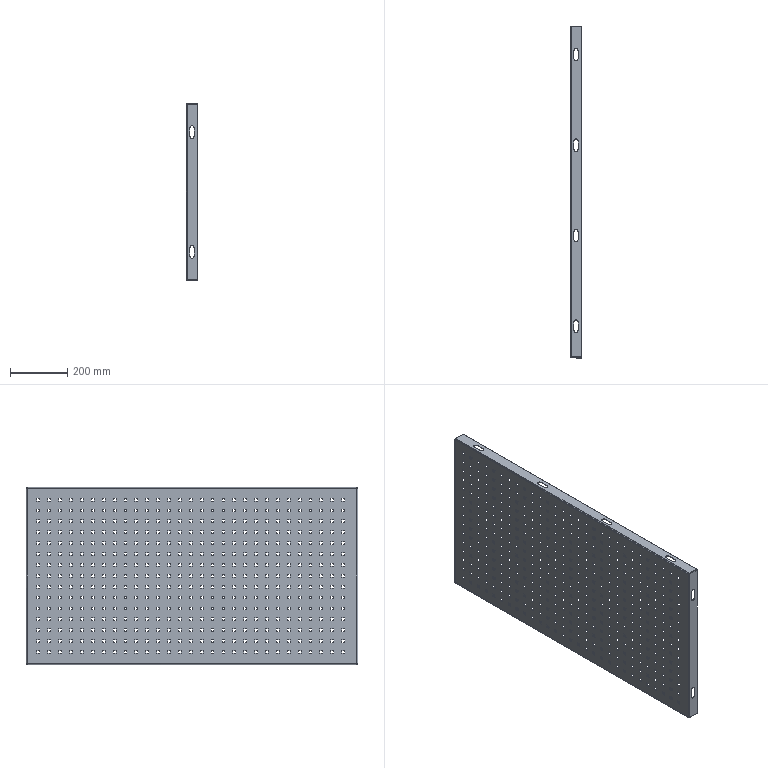Part | SolidWorks | features ICE 3, LPattern 3, EdgeFlange 1, FlatPattern 1, SMBaseFlange 1, SheetMetal 1 | 1 solid | 1826 faces | box 40 x 1158 x 618 mm | volume 1589634 mm3 | plane 1786 | cylinder 32 | spline 8 | commonest cylinder face diameters 14 x24 4 x4 8 x4